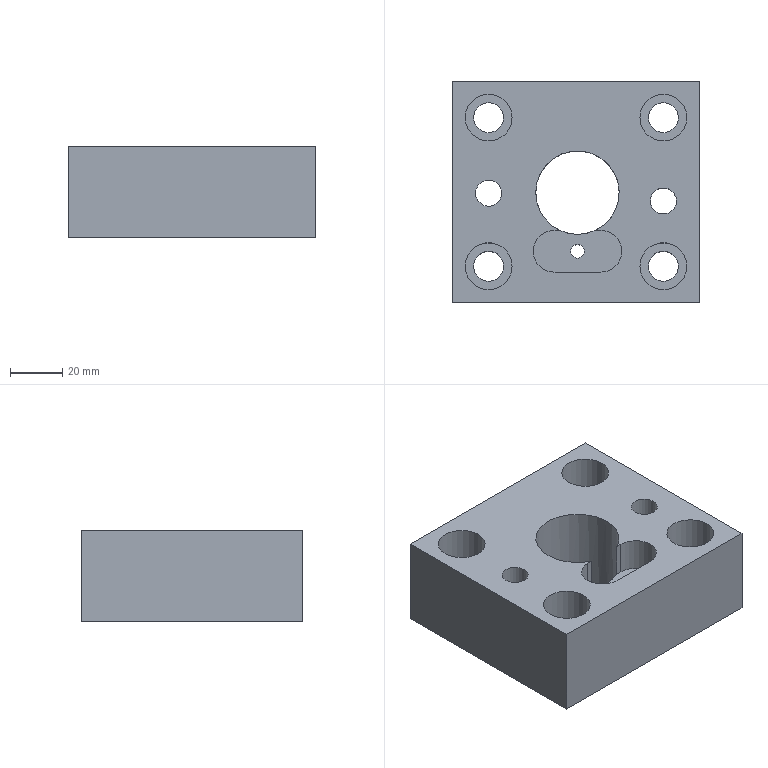Part | STEP file | lll_id4674_x_t | 1 solid | 28 faces | box 95 x 85 x 35 mm | volume 219931 mm3 | plane 14 | cylinder 14 | commonest cylinder face diameters 11.509 x4 18.008 x4 10 x2 16 x2 5.206 x1 32 x1
STEP:
#1=CARTESIAN_POINT('',(434.397,277.5,-35.));
#2=VERTEX_POINT('',#1);
#3=CARTESIAN_POINT('',(437.,277.5,-35.));
#4=DIRECTION('',(0.,0.,1.));
#5=DIRECTION('',(-1.,0.,0.));
#6=AXIS2_PLACEMENT_3D('',#3,#4,#5);
#7=CIRCLE('',#6,2.603);
#8=EDGE_CURVE('',#2,#2,#7,.T.);
#9=ORIENTED_EDGE('',*,*,#8,.T.);
#10=EDGE_LOOP('',(#9));
#11=FACE_BOUND('',#10,.T.);
#12=CARTESIAN_POINT('',(421.,300.,-35.));
#13=VERTEX_POINT('',#12);
#14=CARTESIAN_POINT('',(437.,300.,-35.));
#15=DIRECTION('',(0.,0.,1.));
#16=DIRECTION('',(-1.,0.,0.));
#17=AXIS2_PLACEMENT_3D('',#14,#15,#16);
#18=CIRCLE('',#17,16.);
#19=EDGE_CURVE('',#13,#13,#18,.T.);
#20=ORIENTED_EDGE('',*,*,#19,.T.);
#21=EDGE_LOOP('',(#20));
#22=FACE_BOUND('',#21,.T.);
#23=CARTESIAN_POINT('',(388.935,342.75,-35.));
#24=VERTEX_POINT('',#23);
#25=CARTESIAN_POINT('',(388.935,257.75,-35.));
#26=VERTEX_POINT('',#25);
#27=CARTESIAN_POINT('',(388.935,310.25,-35.));
#28=DIRECTION('',(0.,-1.,0.));
#29=VECTOR('',#28,1.);
#30=LINE('',#27,#29);
#31=EDGE_CURVE('',#24,#26,#30,.T.);
#32=ORIENTED_EDGE('',*,*,#31,.F.);
#33=CARTESIAN_POINT('',(483.935,342.75,-35.));
#34=VERTEX_POINT('',#33);
#35=CARTESIAN_POINT('',(466.435,342.75,-35.));
#36=DIRECTION('',(-1.,0.,0.));
#37=VECTOR('',#36,1.);
#38=LINE('',#35,#37);
#39=EDGE_CURVE('',#34,#24,#38,.T.);
#40=ORIENTED_EDGE('',*,*,#39,.F.);
#41=CARTESIAN_POINT('',(483.935,257.75,-35.));
#42=VERTEX_POINT('',#41);
#43=CARTESIAN_POINT('',(483.935,310.25,-35.));
#44=DIRECTION('',(0.,1.,0.));
#45=VECTOR('',#44,1.);
#46=LINE('',#43,#45);
#47=EDGE_CURVE('',#42,#34,#46,.T.);
#48=ORIENTED_EDGE('',*,*,#47,.F.);
#49=CARTESIAN_POINT('',(466.435,257.75,-35.));
#50=DIRECTION('',(1.,0.,0.));
#51=VECTOR('',#50,1.);
#52=LINE('',#49,#51);
#53=EDGE_CURVE('',#26,#42,#52,.T.);
#54=ORIENTED_EDGE('',*,*,#53,.F.);
#55=EDGE_LOOP('',(#32,#40,#48,#54));
#56=FACE_BOUND('',#55,.T.);
#57=CARTESIAN_POINT('',(475.69,328.75,-35.));
#58=VERTEX_POINT('',#57);
#59=CARTESIAN_POINT('',(469.935,328.75,-35.));
#60=DIRECTION('',(0.,0.,-1.));
#61=DIRECTION('',(1.,0.,0.));
#62=AXIS2_PLACEMENT_3D('',#59,#60,#61);
#63=CIRCLE('',#62,5.755);
#64=EDGE_CURVE('',#58,#58,#63,.T.);
#65=ORIENTED_EDGE('',*,*,#64,.F.);
#66=EDGE_LOOP('',(#65));
#67=FACE_BOUND('',#66,.T.);
#68=CARTESIAN_POINT('',(475.69,271.75,-35.));
#69=VERTEX_POINT('',#68);
#70=CARTESIAN_POINT('',(469.935,271.75,-35.));
#71=DIRECTION('',(0.,0.,-1.));
#72=DIRECTION('',(1.,0.,0.));
#73=AXIS2_PLACEMENT_3D('',#70,#71,#72);
#74=CIRCLE('',#73,5.755);
#75=EDGE_CURVE('',#69,#69,#74,.T.);
#76=ORIENTED_EDGE('',*,*,#75,.F.);
#77=EDGE_LOOP('',(#76));
#78=FACE_BOUND('',#77,.T.);
#79=CARTESIAN_POINT('',(474.935,296.75,-35.));
#80=VERTEX_POINT('',#79);
#81=CARTESIAN_POINT('',(469.935,296.75,-35.));
#82=DIRECTION('',(0.,0.,-1.));
#83=DIRECTION('',(1.,0.,0.));
#84=AXIS2_PLACEMENT_3D('',#81,#82,#83);
#85=CIRCLE('',#84,5.);
#86=EDGE_CURVE('',#80,#80,#85,.T.);
#87=ORIENTED_EDGE('',*,*,#86,.F.);
#88=EDGE_LOOP('',(#87));
#89=FACE_BOUND('',#88,.T.);
#90=CARTESIAN_POINT('',(408.69,271.75,-35.));
#91=VERTEX_POINT('',#90);
#92=CARTESIAN_POINT('',(402.935,271.75,-35.));
#93=DIRECTION('',(0.,0.,-1.));
#94=DIRECTION('',(1.,0.,0.));
#95=AXIS2_PLACEMENT_3D('',#92,#93,#94);
#96=CIRCLE('',#95,5.755);
#97=EDGE_CURVE('',#91,#91,#96,.T.);
#98=ORIENTED_EDGE('',*,*,#97,.F.);
#99=EDGE_LOOP('',(#98));
#100=FACE_BOUND('',#99,.T.);
#101=CARTESIAN_POINT('',(408.69,328.75,-35.));
#102=VERTEX_POINT('',#101);
#103=CARTESIAN_POINT('',(402.935,328.75,-35.));
#104=DIRECTION('',(0.,0.,-1.));
#105=DIRECTION('',(1.,0.,0.));
#106=AXIS2_PLACEMENT_3D('',#103,#104,#105);
#107=CIRCLE('',#106,5.755);
#108=EDGE_CURVE('',#102,#102,#107,.T.);
#109=ORIENTED_EDGE('',*,*,#108,.F.);
#110=EDGE_LOOP('',(#109));
#111=FACE_BOUND('',#110,.T.);
#112=CARTESIAN_POINT('',(407.935,299.75,-35.));
#113=VERTEX_POINT('',#112);
#114=CARTESIAN_POINT('',(402.935,299.75,-35.));
#115=DIRECTION('',(0.,0.,-1.));
#116=DIRECTION('',(1.,0.,0.));
#117=AXIS2_PLACEMENT_3D('',#114,#115,#116);
#118=CIRCLE('',#117,5.);
#119=EDGE_CURVE('',#113,#113,#118,.T.);
#120=ORIENTED_EDGE('',*,*,#119,.F.);
#121=EDGE_LOOP('',(#120));
#122=FACE_BOUND('',#121,.T.);
#123=CARTESIAN_POINT('',(466.435,325.25,-35.));
#124=DIRECTION('',(0.,0.,-1.));
#125=DIRECTION('',(1.,0.,0.));
#126=AXIS2_PLACEMENT_3D('',#123,#124,#125);
#127=PLANE('',#126);
#128=ADVANCED_FACE('',(#11,#22,#56,#67,#78,#89,#100,#111,#122),#127,.T.);
#129=CARTESIAN_POINT('',(446.,269.5,0.));
#130=VERTEX_POINT('',#129);
#131=CARTESIAN_POINT('',(428.,269.5,0.));
#132=VERTEX_POINT('',#131);
#133=CARTESIAN_POINT('',(466.435,269.5,0.));
#134=DIRECTION('',(-1.,0.,0.));
#135=VECTOR('',#134,1.);
#136=LINE('',#133,#135);
#137=EDGE_CURVE('',#130,#132,#136,.T.);
#138=ORIENTED_EDGE('',*,*,#137,.T.);
#139=CARTESIAN_POINT('',(428.,285.5,0.));
#140=VERTEX_POINT('',#139);
#141=CARTESIAN_POINT('',(428.,277.5,0.));
#142=DIRECTION('',(0.,0.,1.));
#143=DIRECTION('',(1.,0.,0.));
#144=AXIS2_PLACEMENT_3D('',#141,#142,#143);
#145=CIRCLE('',#144,8.);
#146=EDGE_CURVE('',#140,#132,#145,.T.);
#147=ORIENTED_EDGE('',*,*,#146,.F.);
#148=CARTESIAN_POINT('',(430.236,285.5,0.));
#149=VERTEX_POINT('',#148);
#150=CARTESIAN_POINT('',(466.435,285.5,0.));
#151=DIRECTION('',(-1.,0.,0.));
#152=VECTOR('',#151,1.);
#153=LINE('',#150,#152);
#154=EDGE_CURVE('',#149,#140,#153,.T.);
#155=ORIENTED_EDGE('',*,*,#154,.F.);
#156=CARTESIAN_POINT('',(443.764,285.5,0.));
#157=VERTEX_POINT('',#156);
#158=CARTESIAN_POINT('',(437.,300.,0.));
#159=DIRECTION('',(0.,0.,-1.));
#160=DIRECTION('',(-1.,0.,0.));
#161=AXIS2_PLACEMENT_3D('',#158,#159,#160);
#162=CIRCLE('',#161,16.);
#163=EDGE_CURVE('',#149,#157,#162,.T.);
#164=ORIENTED_EDGE('',*,*,#163,.T.);
#165=CARTESIAN_POINT('',(446.,285.5,0.));
#166=VERTEX_POINT('',#165);
#167=CARTESIAN_POINT('',(466.435,285.5,0.));
#168=DIRECTION('',(-1.,0.,0.));
#169=VECTOR('',#168,1.);
#170=LINE('',#167,#169);
#171=EDGE_CURVE('',#166,#157,#170,.T.);
#172=ORIENTED_EDGE('',*,*,#171,.F.);
#173=CARTESIAN_POINT('',(446.,277.5,0.));
#174=DIRECTION('',(0.,0.,-1.));
#175=DIRECTION('',(1.,0.,0.));
#176=AXIS2_PLACEMENT_3D('',#173,#174,#175);
#177=CIRCLE('',#176,8.);
#178=EDGE_CURVE('',#166,#130,#177,.T.);
#179=ORIENTED_EDGE('',*,*,#178,.T.);
#180=EDGE_LOOP('',(#138,#147,#155,#164,#172,#179));
#181=FACE_BOUND('',#180,.T.);
#182=CARTESIAN_POINT('',(397.935,299.75,0.));
#183=VERTEX_POINT('',#182);
#184=CARTESIAN_POINT('',(402.935,299.75,0.));
#185=DIRECTION('',(0.,0.,1.));
#186=DIRECTION('',(-1.,0.,0.));
#187=AXIS2_PLACEMENT_3D('',#184,#185,#186);
#188=CIRCLE('',#187,5.);
#189=EDGE_CURVE('',#183,#183,#188,.T.);
#190=ORIENTED_EDGE('',*,*,#189,.F.);
#191=EDGE_LOOP('',(#190));
#192=FACE_BOUND('',#191,.T.);
#193=CARTESIAN_POINT('',(393.931,271.75,0.));
#194=VERTEX_POINT('',#193);
#195=CARTESIAN_POINT('',(402.935,271.75,0.));
#196=DIRECTION('',(0.,0.,-1.));
#197=DIRECTION('',(-1.,0.,0.));
#198=AXIS2_PLACEMENT_3D('',#195,#196,#197);
#199=CIRCLE('',#198,9.004);
#200=EDGE_CURVE('',#194,#194,#199,.T.);
#201=ORIENTED_EDGE('',*,*,#200,.T.);
#202=EDGE_LOOP('',(#201));
#203=FACE_BOUND('',#202,.T.);
#204=CARTESIAN_POINT('',(464.935,296.75,0.));
#205=VERTEX_POINT('',#204);
#206=CARTESIAN_POINT('',(469.935,296.75,0.));
#207=DIRECTION('',(0.,0.,1.));
#208=DIRECTION('',(-1.,0.,0.));
#209=AXIS2_PLACEMENT_3D('',#206,#207,#208);
#210=CIRCLE('',#209,5.);
#211=EDGE_CURVE('',#205,#205,#210,.T.);
#212=ORIENTED_EDGE('',*,*,#211,.F.);
#213=EDGE_LOOP('',(#212));
#214=FACE_BOUND('',#213,.T.);
#215=CARTESIAN_POINT('',(460.931,328.75,0.));
#216=VERTEX_POINT('',#215);
#217=CARTESIAN_POINT('',(469.935,328.75,0.));
#218=DIRECTION('',(0.,0.,-1.));
#219=DIRECTION('',(-1.,0.,0.));
#220=AXIS2_PLACEMENT_3D('',#217,#218,#219);
#221=CIRCLE('',#220,9.004);
#222=EDGE_CURVE('',#216,#216,#221,.T.);
#223=ORIENTED_EDGE('',*,*,#222,.T.);
#224=EDGE_LOOP('',(#223));
#225=FACE_BOUND('',#224,.T.);
#226=CARTESIAN_POINT('',(388.935,342.75,0.));
#227=VERTEX_POINT('',#226);
#228=CARTESIAN_POINT('',(483.935,342.75,0.));
#229=VERTEX_POINT('',#228);
#230=CARTESIAN_POINT('',(466.435,342.75,0.));
#231=DIRECTION('',(1.,0.,0.));
#232=VECTOR('',#231,1.);
#233=LINE('',#230,#232);
#234=EDGE_CURVE('',#227,#229,#233,.T.);
#235=ORIENTED_EDGE('',*,*,#234,.F.);
#236=CARTESIAN_POINT('',(388.935,257.75,0.));
#237=VERTEX_POINT('',#236);
#238=CARTESIAN_POINT('',(388.935,310.25,0.));
#239=DIRECTION('',(0.,1.,0.));
#240=VECTOR('',#239,1.);
#241=LINE('',#238,#240);
#242=EDGE_CURVE('',#237,#227,#241,.T.);
#243=ORIENTED_EDGE('',*,*,#242,.F.);
#244=CARTESIAN_POINT('',(483.935,257.75,0.));
#245=VERTEX_POINT('',#244);
#246=CARTESIAN_POINT('',(466.435,257.75,0.));
#247=DIRECTION('',(-1.,0.,0.));
#248=VECTOR('',#247,1.);
#249=LINE('',#246,#248);
#250=EDGE_CURVE('',#245,#237,#249,.T.);
#251=ORIENTED_EDGE('',*,*,#250,.F.);
#252=CARTESIAN_POINT('',(483.935,310.25,0.));
#253=DIRECTION('',(0.,-1.,0.));
#254=VECTOR('',#253,1.);
#255=LINE('',#252,#254);
#256=EDGE_CURVE('',#229,#245,#255,.T.);
#257=ORIENTED_EDGE('',*,*,#256,.F.);
#258=EDGE_LOOP('',(#235,#243,#251,#257));
#259=FACE_BOUND('',#258,.T.);
#260=CARTESIAN_POINT('',(460.931,271.75,0.));
#261=VERTEX_POINT('',#260);
#262=CARTESIAN_POINT('',(469.935,271.75,0.));
#263=DIRECTION('',(0.,0.,-1.));
#264=DIRECTION('',(-1.,0.,0.));
#265=AXIS2_PLACEMENT_3D('',#262,#263,#264);
#266=CIRCLE('',#265,9.004);
#267=EDGE_CURVE('',#261,#261,#266,.T.);
#268=ORIENTED_EDGE('',*,*,#267,.T.);
#269=EDGE_LOOP('',(#268));
#270=FACE_BOUND('',#269,.T.);
#271=CARTESIAN_POINT('',(393.931,328.75,0.));
#272=VERTEX_POINT('',#271);
#273=CARTESIAN_POINT('',(402.935,328.75,0.));
#274=DIRECTION('',(0.,0.,-1.));
#275=DIRECTION('',(-1.,0.,0.));
#276=AXIS2_PLACEMENT_3D('',#273,#274,#275);
#277=CIRCLE('',#276,9.004);
#278=EDGE_CURVE('',#272,#272,#277,.T.);
#279=ORIENTED_EDGE('',*,*,#278,.T.);
#280=EDGE_LOOP('',(#279));
#281=FACE_BOUND('',#280,.T.);
#282=CARTESIAN_POINT('',(466.435,325.25,0.));
#283=DIRECTION('',(0.,0.,1.));
#284=DIRECTION('',(-1.,0.,0.));
#285=AXIS2_PLACEMENT_3D('',#282,#283,#284);
#286=PLANE('',#285);
#287=ADVANCED_FACE('',(#181,#192,#203,#214,#225,#259,#270,#281),#286,.T.);
#288=CARTESIAN_POINT('',(388.935,342.75,-32.));
#289=DIRECTION('',(0.,0.,1.));
#290=VECTOR('',#289,1.);
#291=LINE('',#288,#290);
#292=EDGE_CURVE('',#24,#227,#291,.T.);
#293=ORIENTED_EDGE('',*,*,#292,.T.);
#294=ORIENTED_EDGE('',*,*,#234,.T.);
#295=CARTESIAN_POINT('',(483.935,342.75,-32.));
#296=DIRECTION('',(0.,0.,1.));
#297=VECTOR('',#296,1.);
#298=LINE('',#295,#297);
#299=EDGE_CURVE('',#34,#229,#298,.T.);
#300=ORIENTED_EDGE('',*,*,#299,.F.);
#301=ORIENTED_EDGE('',*,*,#39,.T.);
#302=EDGE_LOOP('',(#293,#294,#300,#301));
#303=FACE_OUTER_BOUND('',#302,.T.);
#304=CARTESIAN_POINT('',(466.435,342.75,-32.));
#305=DIRECTION('',(0.,1.,0.));
#306=DIRECTION('',(0.,0.,-1.));
#307=AXIS2_PLACEMENT_3D('',#304,#305,#306);
#308=PLANE('',#307);
#309=ADVANCED_FACE('',(#303),#308,.T.);
#310=ORIENTED_EDGE('',*,*,#299,.T.);
#311=ORIENTED_EDGE('',*,*,#256,.T.);
#312=CARTESIAN_POINT('',(483.935,257.75,-32.));
#313=DIRECTION('',(0.,0.,1.));
#314=VECTOR('',#313,1.);
#315=LINE('',#312,#314);
#316=EDGE_CURVE('',#42,#245,#315,.T.);
#317=ORIENTED_EDGE('',*,*,#316,.F.);
#318=ORIENTED_EDGE('',*,*,#47,.T.);
#319=EDGE_LOOP('',(#310,#311,#317,#318));
#320=FACE_OUTER_BOUND('',#319,.T.);
#321=CARTESIAN_POINT('',(483.935,310.25,-32.));
#322=DIRECTION('',(1.,0.,0.));
#323=DIRECTION('',(0.,0.,1.));
#324=AXIS2_PLACEMENT_3D('',#321,#322,#323);
#325=PLANE('',#324);
#326=ADVANCED_FACE('',(#320),#325,.T.);
#327=ORIENTED_EDGE('',*,*,#316,.T.);
#328=ORIENTED_EDGE('',*,*,#250,.T.);
#329=CARTESIAN_POINT('',(388.935,257.75,-32.));
#330=DIRECTION('',(0.,0.,1.));
#331=VECTOR('',#330,1.);
#332=LINE('',#329,#331);
#333=EDGE_CURVE('',#26,#237,#332,.T.);
#334=ORIENTED_EDGE('',*,*,#333,.F.);
#335=ORIENTED_EDGE('',*,*,#53,.T.);
#336=EDGE_LOOP('',(#327,#328,#334,#335));
#337=FACE_OUTER_BOUND('',#336,.T.);
#338=CARTESIAN_POINT('',(466.435,257.75,-32.));
#339=DIRECTION('',(0.,-1.,0.));
#340=DIRECTION('',(0.,0.,1.));
#341=AXIS2_PLACEMENT_3D('',#338,#339,#340);
#342=PLANE('',#341);
#343=ADVANCED_FACE('',(#337),#342,.T.);
#344=ORIENTED_EDGE('',*,*,#31,.T.);
#345=ORIENTED_EDGE('',*,*,#333,.T.);
#346=ORIENTED_EDGE('',*,*,#242,.T.);
#347=ORIENTED_EDGE('',*,*,#292,.F.);
#348=EDGE_LOOP('',(#344,#345,#346,#347));
#349=FACE_OUTER_BOUND('',#348,.T.);
#350=CARTESIAN_POINT('',(388.935,310.25,-32.));
#351=DIRECTION('',(-1.,0.,0.));
#352=DIRECTION('',(0.,0.,-1.));
#353=AXIS2_PLACEMENT_3D('',#350,#351,#352);
#354=PLANE('',#353);
#355=ADVANCED_FACE('',(#349),#354,.T.);
#356=ORIENTED_EDGE('',*,*,#64,.T.);
#357=EDGE_LOOP('',(#356));
#358=FACE_BOUND('',#357,.T.);
#359=CARTESIAN_POINT('',(475.69,328.75,-13.));
#360=VERTEX_POINT('',#359);
#361=CARTESIAN_POINT('',(469.935,328.75,-13.));
#362=DIRECTION('',(0.,0.,-1.));
#363=DIRECTION('',(1.,0.,0.));
#364=AXIS2_PLACEMENT_3D('',#361,#362,#363);
#365=CIRCLE('',#364,5.755);
#366=EDGE_CURVE('',#360,#360,#365,.T.);
#367=ORIENTED_EDGE('',*,*,#366,.F.);
#368=EDGE_LOOP('',(#367));
#369=FACE_BOUND('',#368,.T.);
#370=CARTESIAN_POINT('',(469.935,328.75,2.));
#371=DIRECTION('',(0.,0.,-1.));
#372=DIRECTION('',(-1.,0.,0.));
#373=AXIS2_PLACEMENT_3D('',#370,#371,#372);
#374=CYLINDRICAL_SURFACE('',#373,5.755);
#375=ADVANCED_FACE('',(#358,#369),#374,.F.);
#376=ORIENTED_EDGE('',*,*,#366,.T.);
#377=EDGE_LOOP('',(#376));
#378=FACE_BOUND('',#377,.T.);
#379=CARTESIAN_POINT('',(460.931,328.75,-13.));
#380=VERTEX_POINT('',#379);
#381=CARTESIAN_POINT('',(469.935,328.75,-13.));
#382=DIRECTION('',(0.,0.,-1.));
#383=DIRECTION('',(-1.,0.,0.));
#384=AXIS2_PLACEMENT_3D('',#381,#382,#383);
#385=CIRCLE('',#384,9.004);
#386=EDGE_CURVE('',#380,#380,#385,.T.);
#387=ORIENTED_EDGE('',*,*,#386,.F.);
#388=EDGE_LOOP('',(#387));
#389=FACE_BOUND('',#388,.T.);
#390=CARTESIAN_POINT('',(469.935,328.75,-13.));
#391=DIRECTION('',(0.,0.,-1.));
#392=DIRECTION('',(1.,0.,0.));
#393=AXIS2_PLACEMENT_3D('',#390,#391,#392);
#394=PLANE('',#393);
#395=ADVANCED_FACE('',(#378,#389),#394,.F.);
#396=ORIENTED_EDGE('',*,*,#386,.T.);
#397=EDGE_LOOP('',(#396));
#398=FACE_BOUND('',#397,.T.);
#399=ORIENTED_EDGE('',*,*,#222,.F.);
#400=EDGE_LOOP('',(#399));
#401=FACE_BOUND('',#400,.T.);
#402=CARTESIAN_POINT('',(469.935,328.75,0.));
#403=DIRECTION('',(0.,0.,-1.));
#404=DIRECTION('',(-1.,0.,0.));
#405=AXIS2_PLACEMENT_3D('',#402,#403,#404);
#406=CYLINDRICAL_SURFACE('',#405,9.004);
#407=ADVANCED_FACE('',(#398,#401),#406,.F.);
#408=ORIENTED_EDGE('',*,*,#75,.T.);
#409=EDGE_LOOP('',(#408));
#410=FACE_BOUND('',#409,.T.);
#411=CARTESIAN_POINT('',(475.69,271.75,-13.));
#412=VERTEX_POINT('',#411);
#413=CARTESIAN_POINT('',(469.935,271.75,-13.));
#414=DIRECTION('',(0.,0.,-1.));
#415=DIRECTION('',(1.,0.,0.));
#416=AXIS2_PLACEMENT_3D('',#413,#414,#415);
#417=CIRCLE('',#416,5.755);
#418=EDGE_CURVE('',#412,#412,#417,.T.);
#419=ORIENTED_EDGE('',*,*,#418,.F.);
#420=EDGE_LOOP('',(#419));
#421=FACE_BOUND('',#420,.T.);
#422=CARTESIAN_POINT('',(469.935,271.75,2.));
#423=DIRECTION('',(0.,0.,-1.));
#424=DIRECTION('',(-1.,0.,0.));
#425=AXIS2_PLACEMENT_3D('',#422,#423,#424);
#426=CYLINDRICAL_SURFACE('',#425,5.755);
#427=ADVANCED_FACE('',(#410,#421),#426,.F.);
#428=ORIENTED_EDGE('',*,*,#418,.T.);
#429=EDGE_LOOP('',(#428));
#430=FACE_BOUND('',#429,.T.);
#431=CARTESIAN_POINT('',(460.931,271.75,-13.));
#432=VERTEX_POINT('',#431);
#433=CARTESIAN_POINT('',(469.935,271.75,-13.));
#434=DIRECTION('',(0.,0.,-1.));
#435=DIRECTION('',(-1.,0.,0.));
#436=AXIS2_PLACEMENT_3D('',#433,#434,#435);
#437=CIRCLE('',#436,9.004);
#438=EDGE_CURVE('',#432,#432,#437,.T.);
#439=ORIENTED_EDGE('',*,*,#438,.F.);
#440=EDGE_LOOP('',(#439));
#441=FACE_BOUND('',#440,.T.);
#442=CARTESIAN_POINT('',(469.935,271.75,-13.));
#443=DIRECTION('',(0.,0.,-1.));
#444=DIRECTION('',(1.,0.,0.));
#445=AXIS2_PLACEMENT_3D('',#442,#443,#444);
#446=PLANE('',#445);
#447=ADVANCED_FACE('',(#430,#441),#446,.F.);
#448=ORIENTED_EDGE('',*,*,#438,.T.);
#449=EDGE_LOOP('',(#448));
#450=FACE_BOUND('',#449,.T.);
#451=ORIENTED_EDGE('',*,*,#267,.F.);
#452=EDGE_LOOP('',(#451));
#453=FACE_BOUND('',#452,.T.);
#454=CARTESIAN_POINT('',(469.935,271.75,0.));
#455=DIRECTION('',(0.,0.,-1.));
#456=DIRECTION('',(-1.,0.,0.));
#457=AXIS2_PLACEMENT_3D('',#454,#455,#456);
#458=CYLINDRICAL_SURFACE('',#457,9.004);
#459=ADVANCED_FACE('',(#450,#453),#458,.F.);
#460=ORIENTED_EDGE('',*,*,#211,.T.);
#461=EDGE_LOOP('',(#460));
#462=FACE_BOUND('',#461,.T.);
#463=ORIENTED_EDGE('',*,*,#86,.T.);
#464=EDGE_LOOP('',(#463));
#465=FACE_BOUND('',#464,.T.);
#466=CARTESIAN_POINT('',(469.935,296.75,2.));
#467=DIRECTION('',(0.,0.,-1.));
#468=DIRECTION('',(-1.,0.,0.));
#469=AXIS2_PLACEMENT_3D('',#466,#467,#468);
#470=CYLINDRICAL_SURFACE('',#469,5.);
#471=ADVANCED_FACE('',(#462,#465),#470,.F.);
#472=ORIENTED_EDGE('',*,*,#97,.T.);
#473=EDGE_LOOP('',(#472));
#474=FACE_BOUND('',#473,.T.);
#475=CARTESIAN_POINT('',(408.69,271.75,-13.));
#476=VERTEX_POINT('',#475);
#477=CARTESIAN_POINT('',(402.935,271.75,-13.));
#478=DIRECTION('',(0.,0.,-1.));
#479=DIRECTION('',(1.,0.,0.));
#480=AXIS2_PLACEMENT_3D('',#477,#478,#479);
#481=CIRCLE('',#480,5.755);
#482=EDGE_CURVE('',#476,#476,#481,.T.);
#483=ORIENTED_EDGE('',*,*,#482,.F.);
#484=EDGE_LOOP('',(#483));
#485=FACE_BOUND('',#484,.T.);
#486=CARTESIAN_POINT('',(402.935,271.75,2.));
#487=DIRECTION('',(0.,0.,-1.));
#488=DIRECTION('',(-1.,0.,0.));
#489=AXIS2_PLACEMENT_3D('',#486,#487,#488);
#490=CYLINDRICAL_SURFACE('',#489,5.755);
#491=ADVANCED_FACE('',(#474,#485),#490,.F.);
#492=ORIENTED_EDGE('',*,*,#482,.T.);
#493=EDGE_LOOP('',(#492));
#494=FACE_BOUND('',#493,.T.);
#495=CARTESIAN_POINT('',(393.931,271.75,-13.));
#496=VERTEX_POINT('',#495);
#497=CARTESIAN_POINT('',(402.935,271.75,-13.));
#498=DIRECTION('',(0.,0.,-1.));
#499=DIRECTION('',(-1.,0.,0.));
#500=AXIS2_PLACEMENT_3D('',#497,#498,#499);
#501=CIRCLE('',#500,9.004);
#502=EDGE_CURVE('',#496,#496,#501,.T.);
#503=ORIENTED_EDGE('',*,*,#502,.F.);
#504=EDGE_LOOP('',(#503));
#505=FACE_BOUND('',#504,.T.);
#506=CARTESIAN_POINT('',(402.935,271.75,-13.));
#507=DIRECTION('',(0.,0.,-1.));
#508=DIRECTION('',(1.,0.,0.));
#509=AXIS2_PLACEMENT_3D('',#506,#507,#508);
#510=PLANE('',#509);
#511=ADVANCED_FACE('',(#494,#505),#510,.F.);
#512=ORIENTED_EDGE('',*,*,#502,.T.);
#513=EDGE_LOOP('',(#512));
#514=FACE_BOUND('',#513,.T.);
#515=ORIENTED_EDGE('',*,*,#200,.F.);
#516=EDGE_LOOP('',(#515));
#517=FACE_BOUND('',#516,.T.);
#518=CARTESIAN_POINT('',(402.935,271.75,0.));
#519=DIRECTION('',(0.,0.,-1.));
#520=DIRECTION('',(-1.,0.,0.));
#521=AXIS2_PLACEMENT_3D('',#518,#519,#520);
#522=CYLINDRICAL_SURFACE('',#521,9.004);
#523=ADVANCED_FACE('',(#514,#517),#522,.F.);
#524=ORIENTED_EDGE('',*,*,#108,.T.);
#525=EDGE_LOOP('',(#524));
#526=FACE_BOUND('',#525,.T.);
#527=CARTESIAN_POINT('',(408.69,328.75,-13.));
#528=VERTEX_POINT('',#527);
#529=CARTESIAN_POINT('',(402.935,328.75,-13.));
#530=DIRECTION('',(0.,0.,-1.));
#531=DIRECTION('',(1.,0.,0.));
#532=AXIS2_PLACEMENT_3D('',#529,#530,#531);
#533=CIRCLE('',#532,5.755);
#534=EDGE_CURVE('',#528,#528,#533,.T.);
#535=ORIENTED_EDGE('',*,*,#534,.F.);
#536=EDGE_LOOP('',(#535));
#537=FACE_BOUND('',#536,.T.);
#538=CARTESIAN_POINT('',(402.935,328.75,2.));
#539=DIRECTION('',(0.,0.,-1.));
#540=DIRECTION('',(-1.,0.,0.));
#541=AXIS2_PLACEMENT_3D('',#538,#539,#540);
#542=CYLINDRICAL_SURFACE('',#541,5.755);
#543=ADVANCED_FACE('',(#526,#537),#542,.F.);
#544=ORIENTED_EDGE('',*,*,#534,.T.);
#545=EDGE_LOOP('',(#544));
#546=FACE_BOUND('',#545,.T.);
#547=CARTESIAN_POINT('',(393.931,328.75,-13.));
#548=VERTEX_POINT('',#547);
#549=CARTESIAN_POINT('',(402.935,328.75,-13.));
#550=DIRECTION('',(0.,0.,-1.));
#551=DIRECTION('',(-1.,0.,0.));
#552=AXIS2_PLACEMENT_3D('',#549,#550,#551);
#553=CIRCLE('',#552,9.004);
#554=EDGE_CURVE('',#548,#548,#553,.T.);
#555=ORIENTED_EDGE('',*,*,#554,.F.);
#556=EDGE_LOOP('',(#555));
#557=FACE_BOUND('',#556,.T.);
#558=CARTESIAN_POINT('',(402.935,328.75,-13.));
#559=DIRECTION('',(0.,0.,-1.));
#560=DIRECTION('',(1.,0.,0.));
#561=AXIS2_PLACEMENT_3D('',#558,#559,#560);
#562=PLANE('',#561);
#563=ADVANCED_FACE('',(#546,#557),#562,.F.);
#564=ORIENTED_EDGE('',*,*,#554,.T.);
#565=EDGE_LOOP('',(#564));
#566=FACE_BOUND('',#565,.T.);
#567=ORIENTED_EDGE('',*,*,#278,.F.);
#568=EDGE_LOOP('',(#567));
#569=FACE_BOUND('',#568,.T.);
#570=CARTESIAN_POINT('',(402.935,328.75,0.));
#571=DIRECTION('',(0.,0.,-1.));
#572=DIRECTION('',(-1.,0.,0.));
#573=AXIS2_PLACEMENT_3D('',#570,#571,#572);
#574=CYLINDRICAL_SURFACE('',#573,9.004);
#575=ADVANCED_FACE('',(#566,#569),#574,.F.);
#576=ORIENTED_EDGE('',*,*,#189,.T.);
#577=EDGE_LOOP('',(#576));
#578=FACE_BOUND('',#577,.T.);
#579=ORIENTED_EDGE('',*,*,#119,.T.);
#580=EDGE_LOOP('',(#579));
#581=FACE_BOUND('',#580,.T.);
#582=CARTESIAN_POINT('',(402.935,299.75,2.));
#583=DIRECTION('',(0.,0.,-1.));
#584=DIRECTION('',(-1.,0.,0.));
#585=AXIS2_PLACEMENT_3D('',#582,#583,#584);
#586=CYLINDRICAL_SURFACE('',#585,5.);
#587=ADVANCED_FACE('',(#578,#581),#586,.F.);
#588=ORIENTED_EDGE('',*,*,#8,.F.);
#589=EDGE_LOOP('',(#588));
#590=FACE_BOUND('',#589,.T.);
#591=CARTESIAN_POINT('',(439.603,277.5,-13.));
#592=VERTEX_POINT('',#591);
#593=CARTESIAN_POINT('',(437.,277.5,-13.));
#594=DIRECTION('',(0.,0.,-1.));
#595=DIRECTION('',(1.,0.,0.));
#596=AXIS2_PLACEMENT_3D('',#593,#594,#595);
#597=CIRCLE('',#596,2.603);
#598=EDGE_CURVE('',#592,#592,#597,.T.);
#599=ORIENTED_EDGE('',*,*,#598,.F.);
#600=EDGE_LOOP('',(#599));
#601=FACE_BOUND('',#600,.T.);
#602=CARTESIAN_POINT('',(437.,277.5,-13.));
#603=DIRECTION('',(0.,0.,-1.));
#604=DIRECTION('',(1.,0.,0.));
#605=AXIS2_PLACEMENT_3D('',#602,#603,#604);
#606=CYLINDRICAL_SURFACE('',#605,2.603);
#607=ADVANCED_FACE('',(#590,#601),#606,.F.);
#608=CARTESIAN_POINT('',(428.,285.5,-13.));
#609=VERTEX_POINT('',#608);
#610=CARTESIAN_POINT('',(428.,285.5,-1.));
#611=DIRECTION('',(0.,0.,-1.));
#612=VECTOR('',#611,1.);
#613=LINE('',#610,#612);
#614=EDGE_CURVE('',#140,#609,#613,.T.);
#615=ORIENTED_EDGE('',*,*,#614,.T.);
#616=CARTESIAN_POINT('',(430.236,285.5,-13.));
#617=VERTEX_POINT('',#616);
#618=CARTESIAN_POINT('',(428.,285.5,-13.));
#619=DIRECTION('',(-1.,0.,0.));
#620=VECTOR('',#619,1.);
#621=LINE('',#618,#620);
#622=EDGE_CURVE('',#617,#609,#621,.T.);
#623=ORIENTED_EDGE('',*,*,#622,.F.);
#624=CARTESIAN_POINT('',(430.236,285.5,-15.));
#625=DIRECTION('',(0.,0.,1.));
#626=VECTOR('',#625,1.);
#627=LINE('',#624,#626);
#628=EDGE_CURVE('',#617,#149,#627,.T.);
#629=ORIENTED_EDGE('',*,*,#628,.T.);
#630=ORIENTED_EDGE('',*,*,#154,.T.);
#631=EDGE_LOOP('',(#615,#623,#629,#630));
#632=FACE_OUTER_BOUND('',#631,.T.);
#633=CARTESIAN_POINT('',(0.,285.5,0.));
#634=DIRECTION('',(0.,-1.,0.));
#635=DIRECTION('',(0.,0.,-1.));
#636=AXIS2_PLACEMENT_3D('',#633,#634,#635);
#637=PLANE('',#636);
#638=ADVANCED_FACE('',(#632),#637,.T.);
#639=ORIENTED_EDGE('',*,*,#178,.F.);
#640=CARTESIAN_POINT('',(446.,285.5,-13.));
#641=VERTEX_POINT('',#640);
#642=CARTESIAN_POINT('',(446.,285.5,-7.));
#643=DIRECTION('',(0.,0.,1.));
#644=VECTOR('',#643,1.);
#645=LINE('',#642,#644);
#646=EDGE_CURVE('',#641,#166,#645,.T.);
#647=ORIENTED_EDGE('',*,*,#646,.F.);
#648=CARTESIAN_POINT('',(446.,269.5,-13.));
#649=VERTEX_POINT('',#648);
#650=CARTESIAN_POINT('',(446.,277.5,-13.));
#651=DIRECTION('',(0.,0.,-1.));
#652=DIRECTION('',(1.,0.,0.));
#653=AXIS2_PLACEMENT_3D('',#650,#651,#652);
#654=CIRCLE('',#653,8.);
#655=EDGE_CURVE('',#641,#649,#654,.T.);
#656=ORIENTED_EDGE('',*,*,#655,.T.);
#657=CARTESIAN_POINT('',(446.,269.5,-1.));
#658=DIRECTION('',(0.,0.,1.));
#659=VECTOR('',#658,1.);
#660=LINE('',#657,#659);
#661=EDGE_CURVE('',#649,#130,#660,.T.);
#662=ORIENTED_EDGE('',*,*,#661,.T.);
#663=EDGE_LOOP('',(#639,#647,#656,#662));
#664=FACE_OUTER_BOUND('',#663,.T.);
#665=CARTESIAN_POINT('',(446.,277.5,-1.));
#666=DIRECTION('',(0.,0.,-1.));
#667=DIRECTION('',(1.,0.,0.));
#668=AXIS2_PLACEMENT_3D('',#665,#666,#667);
#669=CYLINDRICAL_SURFACE('',#668,8.);
#670=ADVANCED_FACE('',(#664),#669,.F.);
#671=ORIENTED_EDGE('',*,*,#137,.F.);
#672=ORIENTED_EDGE('',*,*,#661,.F.);
#673=CARTESIAN_POINT('',(428.,269.5,-13.));
#674=VERTEX_POINT('',#673);
#675=CARTESIAN_POINT('',(428.,269.5,-13.));
#676=DIRECTION('',(-1.,0.,0.));
#677=VECTOR('',#676,1.);
#678=LINE('',#675,#677);
#679=EDGE_CURVE('',#649,#674,#678,.T.);
#680=ORIENTED_EDGE('',*,*,#679,.T.);
#681=CARTESIAN_POINT('',(428.,269.5,-1.));
#682=DIRECTION('',(0.,0.,-1.));
#683=VECTOR('',#682,1.);
#684=LINE('',#681,#683);
#685=EDGE_CURVE('',#132,#674,#684,.T.);
#686=ORIENTED_EDGE('',*,*,#685,.F.);
#687=EDGE_LOOP('',(#671,#672,#680,#686));
#688=FACE_OUTER_BOUND('',#687,.T.);
#689=CARTESIAN_POINT('',(0.,269.5,0.));
#690=DIRECTION('',(0.,-1.,0.));
#691=DIRECTION('',(0.,0.,-1.));
#692=AXIS2_PLACEMENT_3D('',#689,#690,#691);
#693=PLANE('',#692);
#694=ADVANCED_FACE('',(#688),#693,.F.);
#695=CARTESIAN_POINT('',(443.764,285.5,-13.));
#696=VERTEX_POINT('',#695);
#697=CARTESIAN_POINT('',(437.,300.,-13.));
#698=DIRECTION('',(0.,0.,-1.));
#699=DIRECTION('',(1.,0.,0.));
#700=AXIS2_PLACEMENT_3D('',#697,#698,#699);
#701=CIRCLE('',#700,16.);
#702=EDGE_CURVE('',#696,#617,#701,.T.);
#703=ORIENTED_EDGE('',*,*,#702,.T.);
#704=ORIENTED_EDGE('',*,*,#622,.T.);
#705=CARTESIAN_POINT('',(428.,277.5,-13.));
#706=DIRECTION('',(0.,0.,-1.));
#707=DIRECTION('',(1.,0.,0.));
#708=AXIS2_PLACEMENT_3D('',#705,#706,#707);
#709=CIRCLE('',#708,8.);
#710=EDGE_CURVE('',#674,#609,#709,.T.);
#711=ORIENTED_EDGE('',*,*,#710,.F.);
#712=ORIENTED_EDGE('',*,*,#679,.F.);
#713=ORIENTED_EDGE('',*,*,#655,.F.);
#714=CARTESIAN_POINT('',(428.,285.5,-13.));
#715=DIRECTION('',(-1.,0.,0.));
#716=VECTOR('',#715,1.);
#717=LINE('',#714,#716);
#718=EDGE_CURVE('',#641,#696,#717,.T.);
#719=ORIENTED_EDGE('',*,*,#718,.T.);
#720=EDGE_LOOP('',(#703,#704,#711,#712,#713,#719));
#721=FACE_BOUND('',#720,.T.);
#722=ORIENTED_EDGE('',*,*,#598,.T.);
#723=EDGE_LOOP('',(#722));
#724=FACE_BOUND('',#723,.T.);
#725=CARTESIAN_POINT('',(428.,277.5,-13.));
#726=DIRECTION('',(0.,0.,1.));
#727=DIRECTION('',(1.,0.,0.));
#728=AXIS2_PLACEMENT_3D('',#725,#726,#727);
#729=PLANE('',#728);
#730=ADVANCED_FACE('',(#721,#724),#729,.T.);
#731=ORIENTED_EDGE('',*,*,#146,.T.);
#732=ORIENTED_EDGE('',*,*,#685,.T.);
#733=ORIENTED_EDGE('',*,*,#710,.T.);
#734=ORIENTED_EDGE('',*,*,#614,.F.);
#735=EDGE_LOOP('',(#731,#732,#733,#734));
#736=FACE_OUTER_BOUND('',#735,.T.);
#737=CARTESIAN_POINT('',(428.,277.5,-1.));
#738=DIRECTION('',(0.,0.,-1.));
#739=DIRECTION('',(1.,0.,0.));
#740=AXIS2_PLACEMENT_3D('',#737,#738,#739);
#741=CYLINDRICAL_SURFACE('',#740,8.);
#742=ADVANCED_FACE('',(#736),#741,.F.);
#743=CARTESIAN_POINT('',(443.764,285.5,-15.));
#744=DIRECTION('',(0.,0.,-1.));
#745=VECTOR('',#744,1.);
#746=LINE('',#743,#745);
#747=EDGE_CURVE('',#157,#696,#746,.T.);
#748=ORIENTED_EDGE('',*,*,#747,.T.);
#749=ORIENTED_EDGE('',*,*,#718,.F.);
#750=ORIENTED_EDGE('',*,*,#646,.T.);
#751=ORIENTED_EDGE('',*,*,#171,.T.);
#752=EDGE_LOOP('',(#748,#749,#750,#751));
#753=FACE_OUTER_BOUND('',#752,.T.);
#754=CARTESIAN_POINT('',(0.,285.5,0.));
#755=DIRECTION('',(0.,-1.,0.));
#756=DIRECTION('',(0.,0.,-1.));
#757=AXIS2_PLACEMENT_3D('',#754,#755,#756);
#758=PLANE('',#757);
#759=ADVANCED_FACE('',(#753),#758,.T.);
#760=ORIENTED_EDGE('',*,*,#628,.F.);
#761=ORIENTED_EDGE('',*,*,#702,.F.);
#762=ORIENTED_EDGE('',*,*,#747,.F.);
#763=ORIENTED_EDGE('',*,*,#163,.F.);
#764=EDGE_LOOP('',(#760,#761,#762,#763));
#765=FACE_BOUND('',#764,.T.);
#766=ORIENTED_EDGE('',*,*,#19,.F.);
#767=EDGE_LOOP('',(#766));
#768=FACE_BOUND('',#767,.T.);
#769=CARTESIAN_POINT('',(437.,300.,-15.));
#770=DIRECTION('',(0.,0.,-1.));
#771=DIRECTION('',(0.,1.,0.));
#772=AXIS2_PLACEMENT_3D('',#769,#770,#771);
#773=CYLINDRICAL_SURFACE('',#772,16.);
#774=ADVANCED_FACE('',(#765,#768),#773,.F.);
#775=CLOSED_SHELL('',(#128,#287,#309,#326,#343,#355,#375,#395,#407,#427,#447,#459,#471,#491,#511,#523,#543,#563,#575,#587,#607,#638,#670,#694,#730,#742,#759,#774));
#776=MANIFOLD_SOLID_BREP('',#775);
#777=(LENGTH_UNIT()NAMED_UNIT(*)SI_UNIT(.MILLI.,.METRE.));
#778=UNCERTAINTY_MEASURE_WITH_UNIT(LENGTH_MEASURE(0.00002),#777,'','');
#779=(NAMED_UNIT(*)PLANE_ANGLE_UNIT()SI_UNIT($,.RADIAN.));
#780=PLANE_ANGLE_MEASURE_WITH_UNIT(PLANE_ANGLE_MEASURE(0.01745),#779);
#781=DIMENSIONAL_EXPONENTS(0.,0.,0.,0.,0.,0.,0.);
#782=(CONVERSION_BASED_UNIT('DEGREE',#780)NAMED_UNIT(#781)PLANE_ANGLE_UNIT());
#783=(NAMED_UNIT(*)SI_UNIT($,.STERADIAN.)SOLID_ANGLE_UNIT());
#784=(GEOMETRIC_REPRESENTATION_CONTEXT(3)GLOBAL_UNCERTAINTY_ASSIGNED_CONTEXT((#778))GLOBAL_UNIT_ASSIGNED_CONTEXT((#777,#782,#783))REPRESENTATION_CONTEXT('',''));
#785=ADVANCED_BREP_SHAPE_REPRESENTATION('',(#776),#784);